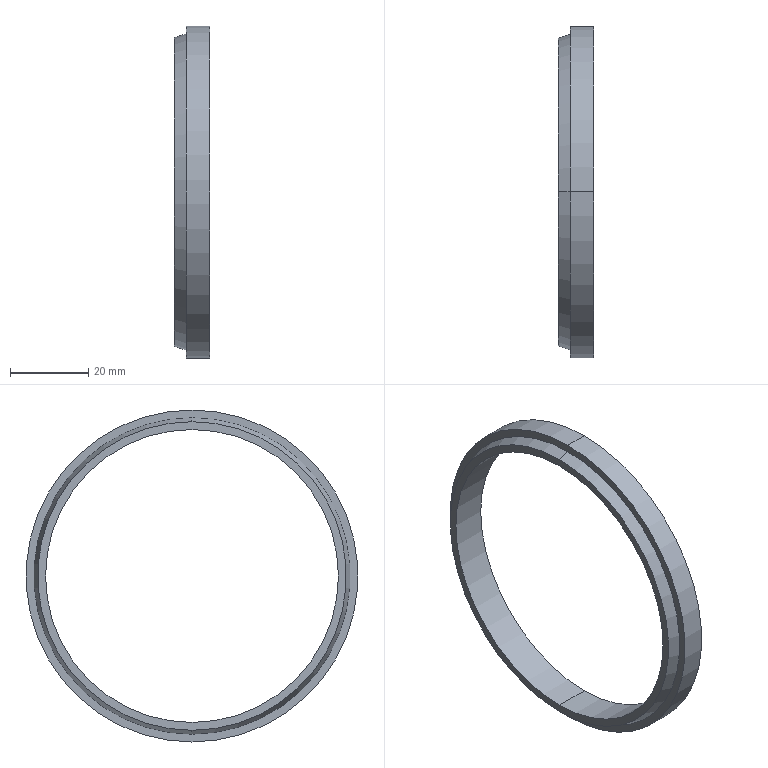Part | SolidWorks | features Revolution 1 | 1 solid | 9 faces | box 9 x 85 x 85 mm | volume 9367 mm3 | cylinder 4 | plane 3 | cone 2 | commonest cylinder face diameters 75 x2 85 x2
STEP:
#1=CARTESIAN_POINT('',(0.,0.,39.5));
#2=VERTEX_POINT('',#1);
#3=CARTESIAN_POINT('',(0.,0.,-39.5));
#4=VERTEX_POINT('',#3);
#5=CARTESIAN_POINT('',(0.,0.,0.));
#6=DIRECTION('',(-1.,0.,0.));
#7=DIRECTION('',(0.,0.,1.));
#8=AXIS2_PLACEMENT_3D('',#5,#6,#7);
#9=CIRCLE('',#8,39.5);
#10=EDGE_CURVE('',#2,#4,#9,.T.);
#11=ORIENTED_EDGE('',*,*,#10,.F.);
#12=CARTESIAN_POINT('',(3.,0.,40.5));
#13=VERTEX_POINT('',#12);
#14=CARTESIAN_POINT('',(3.,0.,40.5));
#15=DIRECTION('',(0.9487,0.,0.3162));
#16=VECTOR('',#15,1000.);
#17=LINE('',#14,#16);
#18=EDGE_CURVE('',#2,#13,#17,.T.);
#19=ORIENTED_EDGE('',*,*,#18,.T.);
#20=CARTESIAN_POINT('',(3.,0.,-40.5));
#21=VERTEX_POINT('',#20);
#22=CARTESIAN_POINT('',(3.,0.,0.));
#23=DIRECTION('',(-1.,0.,0.));
#24=DIRECTION('',(0.,0.,1.));
#25=AXIS2_PLACEMENT_3D('',#22,#23,#24);
#26=CIRCLE('',#25,40.5);
#27=EDGE_CURVE('',#13,#21,#26,.T.);
#28=ORIENTED_EDGE('',*,*,#27,.T.);
#29=CARTESIAN_POINT('',(3.,0.,-40.5));
#30=DIRECTION('',(0.9487,0.,-0.3162));
#31=VECTOR('',#30,1000.);
#32=LINE('',#29,#31);
#33=EDGE_CURVE('',#4,#21,#32,.T.);
#34=ORIENTED_EDGE('',*,*,#33,.F.);
#35=EDGE_LOOP('',(#11,#19,#28,#34));
#36=FACE_OUTER_BOUND('',#35,.T.);
#37=CARTESIAN_POINT('',(3.,0.,0.));
#38=DIRECTION('',(1.,0.,0.));
#39=DIRECTION('',(0.,0.,-1.));
#40=AXIS2_PLACEMENT_3D('',#37,#38,#39);
#41=CONICAL_SURFACE('',#40,40.5,0.3218);
#42=ADVANCED_FACE('',(#36),#41,.T.);
#43=CARTESIAN_POINT('',(9.,0.,42.5));
#44=VERTEX_POINT('',#43);
#45=CARTESIAN_POINT('',(9.,0.,-42.5));
#46=VERTEX_POINT('',#45);
#47=CARTESIAN_POINT('',(9.,0.,0.));
#48=DIRECTION('',(-1.,0.,0.));
#49=DIRECTION('',(0.,0.,1.));
#50=AXIS2_PLACEMENT_3D('',#47,#48,#49);
#51=CIRCLE('',#50,42.5);
#52=EDGE_CURVE('',#44,#46,#51,.T.);
#53=ORIENTED_EDGE('',*,*,#52,.T.);
#54=CARTESIAN_POINT('',(3.,0.,-42.5));
#55=VERTEX_POINT('',#54);
#56=CARTESIAN_POINT('',(-9.114,0.,-42.5));
#57=DIRECTION('',(-1.,0.,0.));
#58=VECTOR('',#57,1000.);
#59=LINE('',#56,#58);
#60=EDGE_CURVE('',#46,#55,#59,.T.);
#61=ORIENTED_EDGE('',*,*,#60,.T.);
#62=CARTESIAN_POINT('',(3.,0.,42.5));
#63=VERTEX_POINT('',#62);
#64=CARTESIAN_POINT('',(3.,0.,0.));
#65=DIRECTION('',(-1.,0.,0.));
#66=DIRECTION('',(0.,0.,1.));
#67=AXIS2_PLACEMENT_3D('',#64,#65,#66);
#68=CIRCLE('',#67,42.5);
#69=EDGE_CURVE('',#63,#55,#68,.T.);
#70=ORIENTED_EDGE('',*,*,#69,.F.);
#71=CARTESIAN_POINT('',(-9.114,0.,42.5));
#72=DIRECTION('',(-1.,0.,0.));
#73=VECTOR('',#72,1000.);
#74=LINE('',#71,#73);
#75=EDGE_CURVE('',#44,#63,#74,.T.);
#76=ORIENTED_EDGE('',*,*,#75,.F.);
#77=EDGE_LOOP('',(#53,#61,#70,#76));
#78=FACE_OUTER_BOUND('',#77,.T.);
#79=CARTESIAN_POINT('',(-9.114,0.,0.));
#80=DIRECTION('',(-1.,0.,0.));
#81=DIRECTION('',(0.,0.,1.));
#82=AXIS2_PLACEMENT_3D('',#79,#80,#81);
#83=CYLINDRICAL_SURFACE('',#82,42.5);
#84=ADVANCED_FACE('',(#78),#83,.T.);
#85=CARTESIAN_POINT('',(9.,0.,-37.5));
#86=VERTEX_POINT('',#85);
#87=CARTESIAN_POINT('',(9.,0.,37.5));
#88=VERTEX_POINT('',#87);
#89=CARTESIAN_POINT('',(9.,0.,0.));
#90=DIRECTION('',(-1.,0.,0.));
#91=DIRECTION('',(0.,0.,1.));
#92=AXIS2_PLACEMENT_3D('',#89,#90,#91);
#93=CIRCLE('',#92,37.5);
#94=EDGE_CURVE('',#86,#88,#93,.T.);
#95=ORIENTED_EDGE('',*,*,#94,.F.);
#96=CARTESIAN_POINT('',(0.,0.,-37.5));
#97=VERTEX_POINT('',#96);
#98=CARTESIAN_POINT('',(-9.114,0.,-37.5));
#99=DIRECTION('',(-1.,0.,0.));
#100=VECTOR('',#99,1000.);
#101=LINE('',#98,#100);
#102=EDGE_CURVE('',#86,#97,#101,.T.);
#103=ORIENTED_EDGE('',*,*,#102,.T.);
#104=CARTESIAN_POINT('',(0.,0.,37.5));
#105=VERTEX_POINT('',#104);
#106=CARTESIAN_POINT('',(0.,0.,0.));
#107=DIRECTION('',(-1.,0.,0.));
#108=DIRECTION('',(0.,0.,1.));
#109=AXIS2_PLACEMENT_3D('',#106,#107,#108);
#110=CIRCLE('',#109,37.5);
#111=EDGE_CURVE('',#97,#105,#110,.T.);
#112=ORIENTED_EDGE('',*,*,#111,.T.);
#113=CARTESIAN_POINT('',(-9.114,0.,37.5));
#114=DIRECTION('',(-1.,0.,0.));
#115=VECTOR('',#114,1000.);
#116=LINE('',#113,#115);
#117=EDGE_CURVE('',#88,#105,#116,.T.);
#118=ORIENTED_EDGE('',*,*,#117,.F.);
#119=EDGE_LOOP('',(#95,#103,#112,#118));
#120=FACE_OUTER_BOUND('',#119,.T.);
#121=CARTESIAN_POINT('',(-9.114,0.,0.));
#122=DIRECTION('',(-1.,0.,0.));
#123=DIRECTION('',(0.,0.,1.));
#124=AXIS2_PLACEMENT_3D('',#121,#122,#123);
#125=CYLINDRICAL_SURFACE('',#124,37.5);
#126=ADVANCED_FACE('',(#120),#125,.F.);
#127=CARTESIAN_POINT('',(0.,0.,0.));
#128=DIRECTION('',(-1.,0.,0.));
#129=DIRECTION('',(0.,0.,1.));
#130=AXIS2_PLACEMENT_3D('',#127,#128,#129);
#131=CIRCLE('',#130,37.5);
#132=EDGE_CURVE('',#105,#97,#131,.T.);
#133=ORIENTED_EDGE('',*,*,#132,.F.);
#134=ORIENTED_EDGE('',*,*,#111,.F.);
#135=EDGE_LOOP('',(#133,#134));
#136=FACE_BOUND('',#135,.T.);
#137=CARTESIAN_POINT('',(0.,0.,0.));
#138=DIRECTION('',(-1.,0.,0.));
#139=DIRECTION('',(0.,0.,1.));
#140=AXIS2_PLACEMENT_3D('',#137,#138,#139);
#141=CIRCLE('',#140,39.5);
#142=EDGE_CURVE('',#4,#2,#141,.T.);
#143=ORIENTED_EDGE('',*,*,#142,.T.);
#144=ORIENTED_EDGE('',*,*,#10,.T.);
#145=EDGE_LOOP('',(#143,#144));
#146=FACE_OUTER_BOUND('',#145,.T.);
#147=CARTESIAN_POINT('',(0.,37.5,0.));
#148=DIRECTION('',(1.,0.,0.));
#149=DIRECTION('',(0.,0.,-1.));
#150=AXIS2_PLACEMENT_3D('',#147,#148,#149);
#151=PLANE('',#150);
#152=ADVANCED_FACE('',(#136,#146),#151,.F.);
#153=ORIENTED_EDGE('',*,*,#102,.F.);
#154=CARTESIAN_POINT('',(9.,0.,0.));
#155=DIRECTION('',(-1.,0.,0.));
#156=DIRECTION('',(0.,0.,1.));
#157=AXIS2_PLACEMENT_3D('',#154,#155,#156);
#158=CIRCLE('',#157,37.5);
#159=EDGE_CURVE('',#88,#86,#158,.T.);
#160=ORIENTED_EDGE('',*,*,#159,.F.);
#161=ORIENTED_EDGE('',*,*,#117,.T.);
#162=ORIENTED_EDGE('',*,*,#132,.T.);
#163=EDGE_LOOP('',(#153,#160,#161,#162));
#164=FACE_OUTER_BOUND('',#163,.T.);
#165=CARTESIAN_POINT('',(-9.114,0.,0.));
#166=DIRECTION('',(-1.,0.,0.));
#167=DIRECTION('',(0.,0.,1.));
#168=AXIS2_PLACEMENT_3D('',#165,#166,#167);
#169=CYLINDRICAL_SURFACE('',#168,37.5);
#170=ADVANCED_FACE('',(#164),#169,.F.);
#171=ORIENTED_EDGE('',*,*,#52,.F.);
#172=CARTESIAN_POINT('',(9.,0.,0.));
#173=DIRECTION('',(-1.,0.,0.));
#174=DIRECTION('',(0.,0.,1.));
#175=AXIS2_PLACEMENT_3D('',#172,#173,#174);
#176=CIRCLE('',#175,42.5);
#177=EDGE_CURVE('',#46,#44,#176,.T.);
#178=ORIENTED_EDGE('',*,*,#177,.F.);
#179=EDGE_LOOP('',(#171,#178));
#180=FACE_OUTER_BOUND('',#179,.T.);
#181=ORIENTED_EDGE('',*,*,#159,.T.);
#182=ORIENTED_EDGE('',*,*,#94,.T.);
#183=EDGE_LOOP('',(#181,#182));
#184=FACE_BOUND('',#183,.T.);
#185=CARTESIAN_POINT('',(9.,37.5,0.));
#186=DIRECTION('',(-1.,0.,0.));
#187=DIRECTION('',(0.,0.,1.));
#188=AXIS2_PLACEMENT_3D('',#185,#186,#187);
#189=PLANE('',#188);
#190=ADVANCED_FACE('',(#180,#184),#189,.F.);
#191=ORIENTED_EDGE('',*,*,#60,.F.);
#192=ORIENTED_EDGE('',*,*,#177,.T.);
#193=ORIENTED_EDGE('',*,*,#75,.T.);
#194=CARTESIAN_POINT('',(3.,0.,0.));
#195=DIRECTION('',(-1.,0.,0.));
#196=DIRECTION('',(0.,0.,1.));
#197=AXIS2_PLACEMENT_3D('',#194,#195,#196);
#198=CIRCLE('',#197,42.5);
#199=EDGE_CURVE('',#55,#63,#198,.T.);
#200=ORIENTED_EDGE('',*,*,#199,.F.);
#201=EDGE_LOOP('',(#191,#192,#193,#200));
#202=FACE_OUTER_BOUND('',#201,.T.);
#203=CARTESIAN_POINT('',(-9.114,0.,0.));
#204=DIRECTION('',(-1.,0.,0.));
#205=DIRECTION('',(0.,0.,1.));
#206=AXIS2_PLACEMENT_3D('',#203,#204,#205);
#207=CYLINDRICAL_SURFACE('',#206,42.5);
#208=ADVANCED_FACE('',(#202),#207,.T.);
#209=CARTESIAN_POINT('',(3.,0.,0.));
#210=DIRECTION('',(-1.,0.,0.));
#211=DIRECTION('',(0.,0.,1.));
#212=AXIS2_PLACEMENT_3D('',#209,#210,#211);
#213=CIRCLE('',#212,40.5);
#214=EDGE_CURVE('',#21,#13,#213,.T.);
#215=ORIENTED_EDGE('',*,*,#214,.F.);
#216=ORIENTED_EDGE('',*,*,#27,.F.);
#217=EDGE_LOOP('',(#215,#216));
#218=FACE_BOUND('',#217,.T.);
#219=ORIENTED_EDGE('',*,*,#69,.T.);
#220=ORIENTED_EDGE('',*,*,#199,.T.);
#221=EDGE_LOOP('',(#219,#220));
#222=FACE_OUTER_BOUND('',#221,.T.);
#223=CARTESIAN_POINT('',(3.,42.5,0.));
#224=DIRECTION('',(1.,0.,0.));
#225=DIRECTION('',(0.,0.,-1.));
#226=AXIS2_PLACEMENT_3D('',#223,#224,#225);
#227=PLANE('',#226);
#228=ADVANCED_FACE('',(#218,#222),#227,.F.);
#229=ORIENTED_EDGE('',*,*,#18,.F.);
#230=ORIENTED_EDGE('',*,*,#142,.F.);
#231=ORIENTED_EDGE('',*,*,#33,.T.);
#232=ORIENTED_EDGE('',*,*,#214,.T.);
#233=EDGE_LOOP('',(#229,#230,#231,#232));
#234=FACE_OUTER_BOUND('',#233,.T.);
#235=CARTESIAN_POINT('',(3.,0.,0.));
#236=DIRECTION('',(1.,0.,0.));
#237=DIRECTION('',(0.,0.,-1.));
#238=AXIS2_PLACEMENT_3D('',#235,#236,#237);
#239=CONICAL_SURFACE('',#238,40.5,0.3218);
#240=ADVANCED_FACE('',(#234),#239,.T.);
#241=CLOSED_SHELL('',(#42,#84,#126,#152,#170,#190,#208,#228,#240));
#242=MANIFOLD_SOLID_BREP('',#241);
#243=CARTESIAN_POINT('',(0.,0.,0.));
#244=DIRECTION('',(0.,0.,1.));
#245=DIRECTION('',(1.,0.,0.));
#246=AXIS2_PLACEMENT_3D('',#243,#244,#245);
#247=(LENGTH_UNIT()NAMED_UNIT(*)SI_UNIT(.MILLI.,.METRE.));
#248=UNCERTAINTY_MEASURE_WITH_UNIT(LENGTH_MEASURE(0.00001),#247,'','');
#249=(NAMED_UNIT(*)PLANE_ANGLE_UNIT()SI_UNIT($,.RADIAN.));
#250=(NAMED_UNIT(*)SI_UNIT($,.STERADIAN.)SOLID_ANGLE_UNIT());
#251=(GEOMETRIC_REPRESENTATION_CONTEXT(3)GLOBAL_UNCERTAINTY_ASSIGNED_CONTEXT((#248))GLOBAL_UNIT_ASSIGNED_CONTEXT((#247,#249,#250))REPRESENTATION_CONTEXT('',''));
#252=ADVANCED_BREP_SHAPE_REPRESENTATION('',(#242,#246),#251);